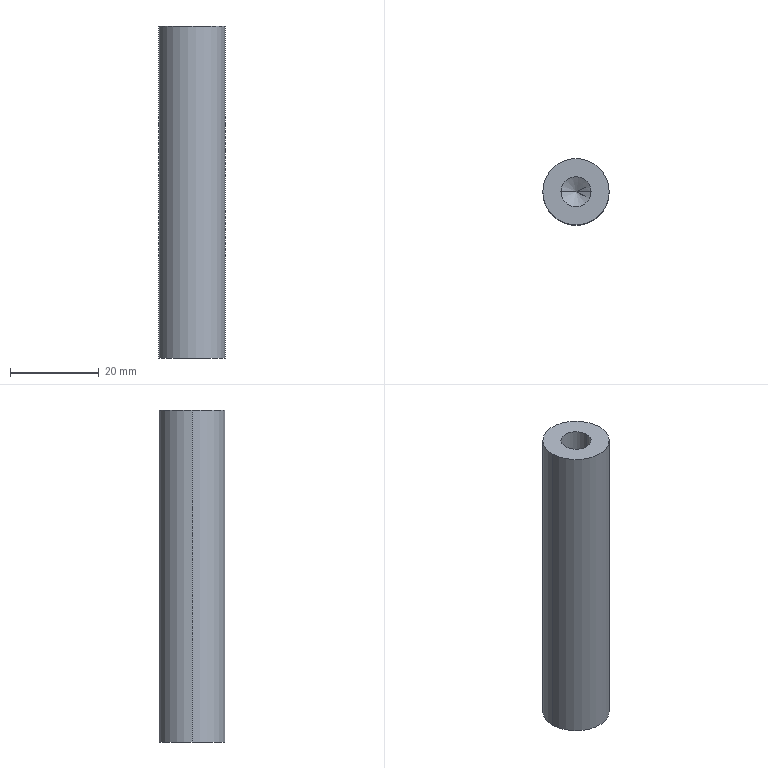Part | SolidWorks | features HoleWzd 2, Extrusion 1 | 1 solid | 12 faces | box 15 x 15 x 75 mm | volume 11770 mm3 | cylinder 6 | cone 4 | plane 2 | commonest cylinder face diameters 6.8 x4 15 x2
STEP:
#1=CARTESIAN_POINT('',(3.4,0.,19.75));
#2=VERTEX_POINT('',#1);
#3=CARTESIAN_POINT('',(-3.4,0.,19.75));
#4=VERTEX_POINT('',#3);
#5=CARTESIAN_POINT('',(0.,0.,19.75));
#6=DIRECTION('',(0.,0.,-1.));
#7=DIRECTION('',(-1.,0.,0.));
#8=AXIS2_PLACEMENT_3D('',#5,#6,#7);
#9=CIRCLE('',#8,3.4);
#10=EDGE_CURVE('',#2,#4,#9,.T.);
#11=ORIENTED_EDGE('',*,*,#10,.F.);
#12=CARTESIAN_POINT('',(3.4,0.,0.));
#13=VERTEX_POINT('',#12);
#14=CARTESIAN_POINT('',(3.4,0.,0.));
#15=DIRECTION('',(0.,0.,-1.));
#16=VECTOR('',#15,1000.);
#17=LINE('',#14,#16);
#18=EDGE_CURVE('',#2,#13,#17,.T.);
#19=ORIENTED_EDGE('',*,*,#18,.T.);
#20=CARTESIAN_POINT('',(-3.4,0.,0.));
#21=VERTEX_POINT('',#20);
#22=CARTESIAN_POINT('',(0.,0.,0.));
#23=DIRECTION('',(0.,0.,-1.));
#24=DIRECTION('',(-1.,0.,0.));
#25=AXIS2_PLACEMENT_3D('',#22,#23,#24);
#26=CIRCLE('',#25,3.4);
#27=EDGE_CURVE('',#13,#21,#26,.T.);
#28=ORIENTED_EDGE('',*,*,#27,.T.);
#29=CARTESIAN_POINT('',(-3.4,0.,0.));
#30=DIRECTION('',(0.,0.,-1.));
#31=VECTOR('',#30,1000.);
#32=LINE('',#29,#31);
#33=EDGE_CURVE('',#4,#21,#32,.T.);
#34=ORIENTED_EDGE('',*,*,#33,.F.);
#35=EDGE_LOOP('',(#11,#19,#28,#34));
#36=FACE_OUTER_BOUND('',#35,.T.);
#37=CARTESIAN_POINT('',(0.,0.,0.));
#38=DIRECTION('',(0.,0.,-1.));
#39=DIRECTION('',(-1.,0.,0.));
#40=AXIS2_PLACEMENT_3D('',#37,#38,#39);
#41=CYLINDRICAL_SURFACE('',#40,3.4);
#42=ADVANCED_FACE('',(#36),#41,.F.);
#43=CARTESIAN_POINT('',(0.,0.,21.793));
#44=VERTEX_POINT('',#43);
#45=CARTESIAN_POINT('',(-3.4,0.,19.75));
#46=DIRECTION('',(-0.8572,0.,-0.515));
#47=VECTOR('',#46,1000.);
#48=LINE('',#45,#47);
#49=EDGE_CURVE('',#44,#4,#48,.T.);
#50=ORIENTED_EDGE('',*,*,#49,.F.);
#51=CARTESIAN_POINT('',(3.4,0.,19.75));
#52=DIRECTION('',(0.8572,0.,-0.515));
#53=VECTOR('',#52,1000.);
#54=LINE('',#51,#53);
#55=EDGE_CURVE('',#44,#2,#54,.T.);
#56=ORIENTED_EDGE('',*,*,#55,.T.);
#57=ORIENTED_EDGE('',*,*,#10,.T.);
#58=EDGE_LOOP('',(#50,#56,#57));
#59=FACE_OUTER_BOUND('',#58,.T.);
#60=CARTESIAN_POINT('',(0.,0.,19.75));
#61=DIRECTION('',(0.,0.,-1.));
#62=DIRECTION('',(-1.,0.,0.));
#63=AXIS2_PLACEMENT_3D('',#60,#61,#62);
#64=CONICAL_SURFACE('',#63,3.4,1.03);
#65=ADVANCED_FACE('',(#59),#64,.F.);
#66=CARTESIAN_POINT('',(-3.4,0.,55.25));
#67=VERTEX_POINT('',#66);
#68=CARTESIAN_POINT('',(3.4,0.,55.25));
#69=VERTEX_POINT('',#68);
#70=CARTESIAN_POINT('',(0.,0.,55.25));
#71=DIRECTION('',(0.,0.,1.));
#72=DIRECTION('',(1.,0.,0.));
#73=AXIS2_PLACEMENT_3D('',#70,#71,#72);
#74=CIRCLE('',#73,3.4);
#75=EDGE_CURVE('',#67,#69,#74,.T.);
#76=ORIENTED_EDGE('',*,*,#75,.F.);
#77=CARTESIAN_POINT('',(-3.4,0.,75.));
#78=VERTEX_POINT('',#77);
#79=CARTESIAN_POINT('',(-3.4,0.,75.));
#80=DIRECTION('',(0.,0.,1.));
#81=VECTOR('',#80,1000.);
#82=LINE('',#79,#81);
#83=EDGE_CURVE('',#67,#78,#82,.T.);
#84=ORIENTED_EDGE('',*,*,#83,.T.);
#85=CARTESIAN_POINT('',(3.4,0.,75.));
#86=VERTEX_POINT('',#85);
#87=CARTESIAN_POINT('',(0.,0.,75.));
#88=DIRECTION('',(0.,0.,1.));
#89=DIRECTION('',(1.,0.,0.));
#90=AXIS2_PLACEMENT_3D('',#87,#88,#89);
#91=CIRCLE('',#90,3.4);
#92=EDGE_CURVE('',#78,#86,#91,.T.);
#93=ORIENTED_EDGE('',*,*,#92,.T.);
#94=CARTESIAN_POINT('',(3.4,0.,75.));
#95=DIRECTION('',(0.,0.,1.));
#96=VECTOR('',#95,1000.);
#97=LINE('',#94,#96);
#98=EDGE_CURVE('',#69,#86,#97,.T.);
#99=ORIENTED_EDGE('',*,*,#98,.F.);
#100=EDGE_LOOP('',(#76,#84,#93,#99));
#101=FACE_OUTER_BOUND('',#100,.T.);
#102=CARTESIAN_POINT('',(0.,0.,75.));
#103=DIRECTION('',(0.,0.,1.));
#104=DIRECTION('',(1.,0.,0.));
#105=AXIS2_PLACEMENT_3D('',#102,#103,#104);
#106=CYLINDRICAL_SURFACE('',#105,3.4);
#107=ADVANCED_FACE('',(#101),#106,.F.);
#108=CARTESIAN_POINT('',(0.,0.,53.207));
#109=VERTEX_POINT('',#108);
#110=CARTESIAN_POINT('',(3.4,0.,55.25));
#111=DIRECTION('',(0.8572,0.,0.515));
#112=VECTOR('',#111,1000.);
#113=LINE('',#110,#112);
#114=EDGE_CURVE('',#109,#69,#113,.T.);
#115=ORIENTED_EDGE('',*,*,#114,.F.);
#116=CARTESIAN_POINT('',(-3.4,0.,55.25));
#117=DIRECTION('',(-0.8572,0.,0.515));
#118=VECTOR('',#117,1000.);
#119=LINE('',#116,#118);
#120=EDGE_CURVE('',#109,#67,#119,.T.);
#121=ORIENTED_EDGE('',*,*,#120,.T.);
#122=ORIENTED_EDGE('',*,*,#75,.T.);
#123=EDGE_LOOP('',(#115,#121,#122));
#124=FACE_OUTER_BOUND('',#123,.T.);
#125=CARTESIAN_POINT('',(0.,0.,55.25));
#126=DIRECTION('',(0.,0.,1.));
#127=DIRECTION('',(1.,0.,0.));
#128=AXIS2_PLACEMENT_3D('',#125,#126,#127);
#129=CONICAL_SURFACE('',#128,3.4,1.03);
#130=ADVANCED_FACE('',(#124),#129,.F.);
#131=CARTESIAN_POINT('',(7.5,0.,75.));
#132=VERTEX_POINT('',#131);
#133=CARTESIAN_POINT('',(-7.5,0.,75.));
#134=VERTEX_POINT('',#133);
#135=CARTESIAN_POINT('',(0.,0.,75.));
#136=DIRECTION('',(0.,0.,1.));
#137=DIRECTION('',(1.,0.,0.));
#138=AXIS2_PLACEMENT_3D('',#135,#136,#137);
#139=CIRCLE('',#138,7.5);
#140=EDGE_CURVE('',#132,#134,#139,.T.);
#141=ORIENTED_EDGE('',*,*,#140,.F.);
#142=CARTESIAN_POINT('',(7.5,0.,0.));
#143=VERTEX_POINT('',#142);
#144=CARTESIAN_POINT('',(7.5,0.,75.));
#145=DIRECTION('',(0.,0.,-1.));
#146=VECTOR('',#145,1000.);
#147=LINE('',#144,#146);
#148=EDGE_CURVE('',#132,#143,#147,.T.);
#149=ORIENTED_EDGE('',*,*,#148,.T.);
#150=CARTESIAN_POINT('',(-7.5,0.,0.));
#151=VERTEX_POINT('',#150);
#152=CARTESIAN_POINT('',(0.,0.,0.));
#153=DIRECTION('',(0.,0.,1.));
#154=DIRECTION('',(1.,0.,0.));
#155=AXIS2_PLACEMENT_3D('',#152,#153,#154);
#156=CIRCLE('',#155,7.5);
#157=EDGE_CURVE('',#143,#151,#156,.T.);
#158=ORIENTED_EDGE('',*,*,#157,.T.);
#159=CARTESIAN_POINT('',(-7.5,0.,75.));
#160=DIRECTION('',(0.,0.,-1.));
#161=VECTOR('',#160,1000.);
#162=LINE('',#159,#161);
#163=EDGE_CURVE('',#134,#151,#162,.T.);
#164=ORIENTED_EDGE('',*,*,#163,.F.);
#165=EDGE_LOOP('',(#141,#149,#158,#164));
#166=FACE_OUTER_BOUND('',#165,.T.);
#167=CARTESIAN_POINT('',(0.,0.,75.));
#168=DIRECTION('',(0.,0.,-1.));
#169=DIRECTION('',(-1.,0.,0.));
#170=AXIS2_PLACEMENT_3D('',#167,#168,#169);
#171=CYLINDRICAL_SURFACE('',#170,7.5);
#172=ADVANCED_FACE('',(#166),#171,.T.);
#173=ORIENTED_EDGE('',*,*,#148,.F.);
#174=CARTESIAN_POINT('',(0.,0.,75.));
#175=DIRECTION('',(0.,0.,1.));
#176=DIRECTION('',(1.,0.,0.));
#177=AXIS2_PLACEMENT_3D('',#174,#175,#176);
#178=CIRCLE('',#177,7.5);
#179=EDGE_CURVE('',#134,#132,#178,.T.);
#180=ORIENTED_EDGE('',*,*,#179,.F.);
#181=ORIENTED_EDGE('',*,*,#163,.T.);
#182=CARTESIAN_POINT('',(0.,0.,0.));
#183=DIRECTION('',(0.,0.,1.));
#184=DIRECTION('',(1.,0.,0.));
#185=AXIS2_PLACEMENT_3D('',#182,#183,#184);
#186=CIRCLE('',#185,7.5);
#187=EDGE_CURVE('',#151,#143,#186,.T.);
#188=ORIENTED_EDGE('',*,*,#187,.T.);
#189=EDGE_LOOP('',(#173,#180,#181,#188));
#190=FACE_OUTER_BOUND('',#189,.T.);
#191=CARTESIAN_POINT('',(0.,0.,75.));
#192=DIRECTION('',(0.,0.,-1.));
#193=DIRECTION('',(-1.,0.,0.));
#194=AXIS2_PLACEMENT_3D('',#191,#192,#193);
#195=CYLINDRICAL_SURFACE('',#194,7.5);
#196=ADVANCED_FACE('',(#190),#195,.T.);
#197=CARTESIAN_POINT('',(0.,0.,75.));
#198=DIRECTION('',(0.,0.,1.));
#199=DIRECTION('',(1.,0.,0.));
#200=AXIS2_PLACEMENT_3D('',#197,#198,#199);
#201=CIRCLE('',#200,3.4);
#202=EDGE_CURVE('',#86,#78,#201,.T.);
#203=ORIENTED_EDGE('',*,*,#202,.F.);
#204=ORIENTED_EDGE('',*,*,#92,.F.);
#205=EDGE_LOOP('',(#203,#204));
#206=FACE_BOUND('',#205,.T.);
#207=ORIENTED_EDGE('',*,*,#179,.T.);
#208=ORIENTED_EDGE('',*,*,#140,.T.);
#209=EDGE_LOOP('',(#207,#208));
#210=FACE_OUTER_BOUND('',#209,.T.);
#211=CARTESIAN_POINT('',(0.,0.,75.));
#212=DIRECTION('',(0.,0.,1.));
#213=DIRECTION('',(1.,0.,0.));
#214=AXIS2_PLACEMENT_3D('',#211,#212,#213);
#215=PLANE('',#214);
#216=ADVANCED_FACE('',(#206,#210),#215,.T.);
#217=CARTESIAN_POINT('',(0.,0.,0.));
#218=DIRECTION('',(0.,0.,-1.));
#219=DIRECTION('',(-1.,0.,0.));
#220=AXIS2_PLACEMENT_3D('',#217,#218,#219);
#221=CIRCLE('',#220,3.4);
#222=EDGE_CURVE('',#21,#13,#221,.T.);
#223=ORIENTED_EDGE('',*,*,#222,.F.);
#224=ORIENTED_EDGE('',*,*,#27,.F.);
#225=EDGE_LOOP('',(#223,#224));
#226=FACE_BOUND('',#225,.T.);
#227=ORIENTED_EDGE('',*,*,#187,.F.);
#228=ORIENTED_EDGE('',*,*,#157,.F.);
#229=EDGE_LOOP('',(#227,#228));
#230=FACE_OUTER_BOUND('',#229,.T.);
#231=CARTESIAN_POINT('',(0.,0.,0.));
#232=DIRECTION('',(0.,0.,1.));
#233=DIRECTION('',(1.,0.,0.));
#234=AXIS2_PLACEMENT_3D('',#231,#232,#233);
#235=PLANE('',#234);
#236=ADVANCED_FACE('',(#226,#230),#235,.F.);
#237=ORIENTED_EDGE('',*,*,#120,.F.);
#238=ORIENTED_EDGE('',*,*,#114,.T.);
#239=CARTESIAN_POINT('',(0.,0.,55.25));
#240=DIRECTION('',(0.,0.,1.));
#241=DIRECTION('',(1.,0.,0.));
#242=AXIS2_PLACEMENT_3D('',#239,#240,#241);
#243=CIRCLE('',#242,3.4);
#244=EDGE_CURVE('',#69,#67,#243,.T.);
#245=ORIENTED_EDGE('',*,*,#244,.T.);
#246=EDGE_LOOP('',(#237,#238,#245));
#247=FACE_OUTER_BOUND('',#246,.T.);
#248=CARTESIAN_POINT('',(0.,0.,55.25));
#249=DIRECTION('',(0.,0.,1.));
#250=DIRECTION('',(1.,0.,0.));
#251=AXIS2_PLACEMENT_3D('',#248,#249,#250);
#252=CONICAL_SURFACE('',#251,3.4,1.03);
#253=ADVANCED_FACE('',(#247),#252,.F.);
#254=ORIENTED_EDGE('',*,*,#83,.F.);
#255=ORIENTED_EDGE('',*,*,#244,.F.);
#256=ORIENTED_EDGE('',*,*,#98,.T.);
#257=ORIENTED_EDGE('',*,*,#202,.T.);
#258=EDGE_LOOP('',(#254,#255,#256,#257));
#259=FACE_OUTER_BOUND('',#258,.T.);
#260=CARTESIAN_POINT('',(0.,0.,75.));
#261=DIRECTION('',(0.,0.,1.));
#262=DIRECTION('',(1.,0.,0.));
#263=AXIS2_PLACEMENT_3D('',#260,#261,#262);
#264=CYLINDRICAL_SURFACE('',#263,3.4);
#265=ADVANCED_FACE('',(#259),#264,.F.);
#266=ORIENTED_EDGE('',*,*,#55,.F.);
#267=ORIENTED_EDGE('',*,*,#49,.T.);
#268=CARTESIAN_POINT('',(0.,0.,19.75));
#269=DIRECTION('',(0.,0.,-1.));
#270=DIRECTION('',(-1.,0.,0.));
#271=AXIS2_PLACEMENT_3D('',#268,#269,#270);
#272=CIRCLE('',#271,3.4);
#273=EDGE_CURVE('',#4,#2,#272,.T.);
#274=ORIENTED_EDGE('',*,*,#273,.T.);
#275=EDGE_LOOP('',(#266,#267,#274));
#276=FACE_OUTER_BOUND('',#275,.T.);
#277=CARTESIAN_POINT('',(0.,0.,19.75));
#278=DIRECTION('',(0.,0.,-1.));
#279=DIRECTION('',(-1.,0.,0.));
#280=AXIS2_PLACEMENT_3D('',#277,#278,#279);
#281=CONICAL_SURFACE('',#280,3.4,1.03);
#282=ADVANCED_FACE('',(#276),#281,.F.);
#283=ORIENTED_EDGE('',*,*,#18,.F.);
#284=ORIENTED_EDGE('',*,*,#273,.F.);
#285=ORIENTED_EDGE('',*,*,#33,.T.);
#286=ORIENTED_EDGE('',*,*,#222,.T.);
#287=EDGE_LOOP('',(#283,#284,#285,#286));
#288=FACE_OUTER_BOUND('',#287,.T.);
#289=CARTESIAN_POINT('',(0.,0.,0.));
#290=DIRECTION('',(0.,0.,-1.));
#291=DIRECTION('',(-1.,0.,0.));
#292=AXIS2_PLACEMENT_3D('',#289,#290,#291);
#293=CYLINDRICAL_SURFACE('',#292,3.4);
#294=ADVANCED_FACE('',(#288),#293,.F.);
#295=CLOSED_SHELL('',(#42,#65,#107,#130,#172,#196,#216,#236,#253,#265,#282,#294));
#296=MANIFOLD_SOLID_BREP('',#295);
#297=CARTESIAN_POINT('',(0.,0.,0.));
#298=DIRECTION('',(0.,0.,1.));
#299=DIRECTION('',(1.,0.,0.));
#300=AXIS2_PLACEMENT_3D('',#297,#298,#299);
#301=(LENGTH_UNIT()NAMED_UNIT(*)SI_UNIT(.MILLI.,.METRE.));
#302=UNCERTAINTY_MEASURE_WITH_UNIT(LENGTH_MEASURE(0.00001),#301,'','');
#303=(NAMED_UNIT(*)PLANE_ANGLE_UNIT()SI_UNIT($,.RADIAN.));
#304=(NAMED_UNIT(*)SI_UNIT($,.STERADIAN.)SOLID_ANGLE_UNIT());
#305=(GEOMETRIC_REPRESENTATION_CONTEXT(3)GLOBAL_UNCERTAINTY_ASSIGNED_CONTEXT((#302))GLOBAL_UNIT_ASSIGNED_CONTEXT((#301,#303,#304))REPRESENTATION_CONTEXT('',''));
#306=ADVANCED_BREP_SHAPE_REPRESENTATION('',(#296,#300),#305);